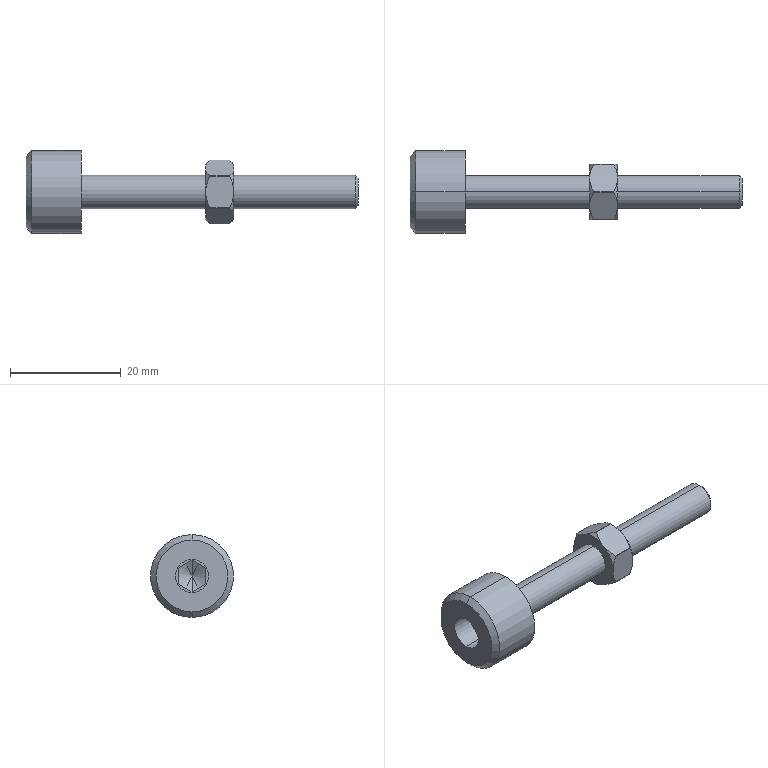Part | STEP file | limit screw Y-JAB22-M6-L50 | 1 solid | 54 faces | box 60 x 15 x 15 mm | volume 3261 mm3 | cone 20 | plane 19 | cylinder 15 | commonest cylinder face diameters 11.5 x7 6 x6 15 x2